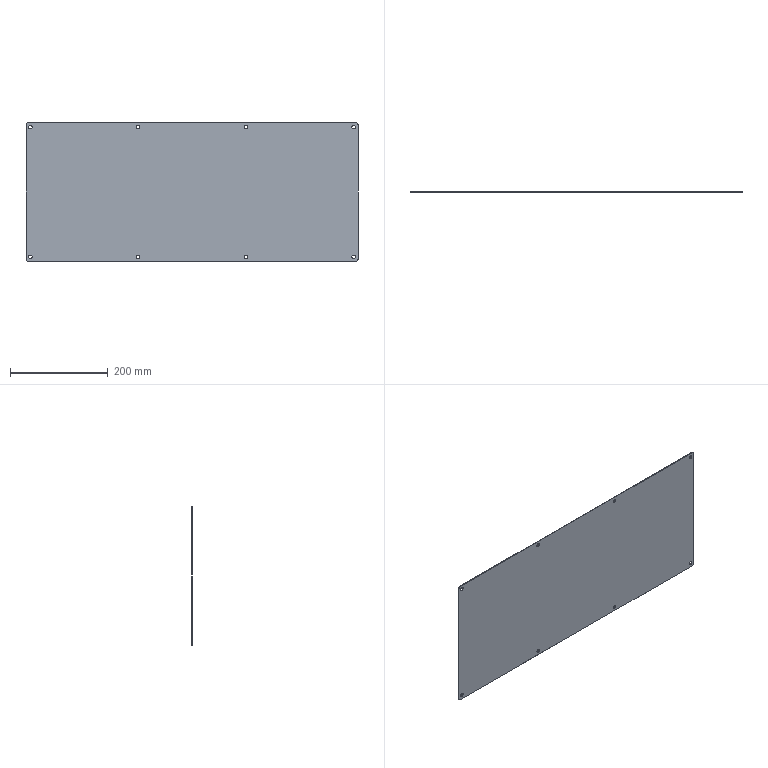Part | NX | features solid 2 | 1 solid | 26 faces | box 678 x 1.5 x 283 mm | volume 287329 mm3 | cylinder 20 | plane 6 | commonest cylinder face diameters 7 x16 8 x4
STEP:
#1=CARTESIAN_POINT('',(-330.,-1319.5,-521.5));
#2=VERTEX_POINT('',#1);
#3=CARTESIAN_POINT('',(-330.,-1318.,-521.5));
#4=VERTEX_POINT('',#3);
#5=CARTESIAN_POINT('',(-330.,-584.806,-521.5));
#6=DIRECTION('',(0.,-1.,0.));
#7=VECTOR('',#6,1000.);
#8=LINE('',#5,#7);
#9=EDGE_CURVE('',#2,#4,#8,.F.);
#10=ORIENTED_EDGE('',*,*,#9,.T.);
#11=CARTESIAN_POINT('',(-330.,-1318.,-528.5));
#12=VERTEX_POINT('',#11);
#13=CARTESIAN_POINT('',(-330.,-1318.,-525.));
#14=DIRECTION('',(0.,1.,0.));
#15=DIRECTION('',(0.,0.,1.));
#16=AXIS2_PLACEMENT_3D('',#13,#14,#15);
#17=CIRCLE('',#16,3.5);
#18=EDGE_CURVE('',#4,#12,#17,.T.);
#19=ORIENTED_EDGE('',*,*,#18,.T.);
#20=CARTESIAN_POINT('',(-330.,-1319.5,-528.5));
#21=VERTEX_POINT('',#20);
#22=CARTESIAN_POINT('',(-330.,-584.806,-528.5));
#23=DIRECTION('',(0.,-1.,0.));
#24=VECTOR('',#23,1000.);
#25=LINE('',#22,#24);
#26=EDGE_CURVE('',#12,#21,#25,.T.);
#27=ORIENTED_EDGE('',*,*,#26,.T.);
#28=CARTESIAN_POINT('',(-330.,-1319.5,-525.));
#29=DIRECTION('',(0.,-1.,0.));
#30=DIRECTION('',(1.,0.,0.));
#31=AXIS2_PLACEMENT_3D('',#28,#29,#30);
#32=CIRCLE('',#31,3.5);
#33=EDGE_CURVE('',#21,#2,#32,.T.);
#34=ORIENTED_EDGE('',*,*,#33,.T.);
#35=EDGE_LOOP('',(#10,#19,#27,#34));
#36=FACE_BOUND('',#35,.T.);
#37=CARTESIAN_POINT('',(-330.,-584.806,-525.));
#38=DIRECTION('',(0.,-1.,0.));
#39=DIRECTION('',(0.,0.,-1.));
#40=AXIS2_PLACEMENT_3D('',#37,#38,#39);
#41=CYLINDRICAL_SURFACE('',#40,3.5);
#42=ADVANCED_FACE('',(#36),#41,.F.);
#43=CARTESIAN_POINT('',(-110.,-1318.,-521.5));
#44=VERTEX_POINT('',#43);
#45=CARTESIAN_POINT('',(-110.,-1319.5,-521.5));
#46=VERTEX_POINT('',#45);
#47=CARTESIAN_POINT('',(-110.,-584.806,-521.5));
#48=DIRECTION('',(0.,-1.,0.));
#49=VECTOR('',#48,1000.);
#50=LINE('',#47,#49);
#51=EDGE_CURVE('',#44,#46,#50,.T.);
#52=ORIENTED_EDGE('',*,*,#51,.F.);
#53=CARTESIAN_POINT('',(-110.,-1318.,-528.5));
#54=VERTEX_POINT('',#53);
#55=CARTESIAN_POINT('',(-110.,-1318.,-525.));
#56=DIRECTION('',(0.,1.,0.));
#57=DIRECTION('',(0.,0.,1.));
#58=AXIS2_PLACEMENT_3D('',#55,#56,#57);
#59=CIRCLE('',#58,3.5);
#60=EDGE_CURVE('',#44,#54,#59,.T.);
#61=ORIENTED_EDGE('',*,*,#60,.T.);
#62=CARTESIAN_POINT('',(-110.,-1319.5,-528.5));
#63=VERTEX_POINT('',#62);
#64=CARTESIAN_POINT('',(-110.,-584.806,-528.5));
#65=DIRECTION('',(0.,-1.,0.));
#66=VECTOR('',#65,1000.);
#67=LINE('',#64,#66);
#68=EDGE_CURVE('',#63,#54,#67,.F.);
#69=ORIENTED_EDGE('',*,*,#68,.F.);
#70=CARTESIAN_POINT('',(-110.,-1319.5,-525.));
#71=DIRECTION('',(0.,-1.,0.));
#72=DIRECTION('',(1.,0.,0.));
#73=AXIS2_PLACEMENT_3D('',#70,#71,#72);
#74=CIRCLE('',#73,3.5);
#75=EDGE_CURVE('',#63,#46,#74,.T.);
#76=ORIENTED_EDGE('',*,*,#75,.T.);
#77=EDGE_LOOP('',(#52,#61,#69,#76));
#78=FACE_BOUND('',#77,.T.);
#79=CARTESIAN_POINT('',(-110.,-584.806,-525.));
#80=DIRECTION('',(0.,-1.,0.));
#81=DIRECTION('',(0.,0.,-1.));
#82=AXIS2_PLACEMENT_3D('',#79,#80,#81);
#83=CYLINDRICAL_SURFACE('',#82,3.5);
#84=ADVANCED_FACE('',(#78),#83,.F.);
#85=CARTESIAN_POINT('',(110.,-1318.,-521.5));
#86=VERTEX_POINT('',#85);
#87=CARTESIAN_POINT('',(110.,-1319.5,-521.5));
#88=VERTEX_POINT('',#87);
#89=CARTESIAN_POINT('',(110.,-584.806,-521.5));
#90=DIRECTION('',(0.,-1.,0.));
#91=VECTOR('',#90,1000.);
#92=LINE('',#89,#91);
#93=EDGE_CURVE('',#86,#88,#92,.T.);
#94=ORIENTED_EDGE('',*,*,#93,.F.);
#95=CARTESIAN_POINT('',(110.,-1318.,-528.5));
#96=VERTEX_POINT('',#95);
#97=CARTESIAN_POINT('',(110.,-1318.,-525.));
#98=DIRECTION('',(0.,1.,0.));
#99=DIRECTION('',(0.,0.,1.));
#100=AXIS2_PLACEMENT_3D('',#97,#98,#99);
#101=CIRCLE('',#100,3.5);
#102=EDGE_CURVE('',#86,#96,#101,.T.);
#103=ORIENTED_EDGE('',*,*,#102,.T.);
#104=CARTESIAN_POINT('',(110.,-1319.5,-528.5));
#105=VERTEX_POINT('',#104);
#106=CARTESIAN_POINT('',(110.,-584.806,-528.5));
#107=DIRECTION('',(0.,-1.,0.));
#108=VECTOR('',#107,1000.);
#109=LINE('',#106,#108);
#110=EDGE_CURVE('',#105,#96,#109,.F.);
#111=ORIENTED_EDGE('',*,*,#110,.F.);
#112=CARTESIAN_POINT('',(110.,-1319.5,-525.));
#113=DIRECTION('',(0.,-1.,0.));
#114=DIRECTION('',(1.,0.,0.));
#115=AXIS2_PLACEMENT_3D('',#112,#113,#114);
#116=CIRCLE('',#115,3.5);
#117=EDGE_CURVE('',#105,#88,#116,.T.);
#118=ORIENTED_EDGE('',*,*,#117,.T.);
#119=EDGE_LOOP('',(#94,#103,#111,#118));
#120=FACE_BOUND('',#119,.T.);
#121=CARTESIAN_POINT('',(110.,-584.806,-525.));
#122=DIRECTION('',(0.,-1.,0.));
#123=DIRECTION('',(0.,0.,-1.));
#124=AXIS2_PLACEMENT_3D('',#121,#122,#123);
#125=CYLINDRICAL_SURFACE('',#124,3.5);
#126=ADVANCED_FACE('',(#120),#125,.F.);
#127=CARTESIAN_POINT('',(330.,-1318.,-521.5));
#128=VERTEX_POINT('',#127);
#129=CARTESIAN_POINT('',(330.,-1319.5,-521.5));
#130=VERTEX_POINT('',#129);
#131=CARTESIAN_POINT('',(330.,-584.806,-521.5));
#132=DIRECTION('',(0.,-1.,0.));
#133=VECTOR('',#132,1000.);
#134=LINE('',#131,#133);
#135=EDGE_CURVE('',#128,#130,#134,.T.);
#136=ORIENTED_EDGE('',*,*,#135,.F.);
#137=CARTESIAN_POINT('',(330.,-1318.,-528.5));
#138=VERTEX_POINT('',#137);
#139=CARTESIAN_POINT('',(330.,-1318.,-525.));
#140=DIRECTION('',(0.,1.,0.));
#141=DIRECTION('',(0.,0.,1.));
#142=AXIS2_PLACEMENT_3D('',#139,#140,#141);
#143=CIRCLE('',#142,3.5);
#144=EDGE_CURVE('',#128,#138,#143,.T.);
#145=ORIENTED_EDGE('',*,*,#144,.T.);
#146=CARTESIAN_POINT('',(330.,-1319.5,-528.5));
#147=VERTEX_POINT('',#146);
#148=CARTESIAN_POINT('',(330.,-584.806,-528.5));
#149=DIRECTION('',(0.,-1.,0.));
#150=VECTOR('',#149,1000.);
#151=LINE('',#148,#150);
#152=EDGE_CURVE('',#147,#138,#151,.F.);
#153=ORIENTED_EDGE('',*,*,#152,.F.);
#154=CARTESIAN_POINT('',(330.,-1319.5,-525.));
#155=DIRECTION('',(0.,-1.,0.));
#156=DIRECTION('',(1.,0.,0.));
#157=AXIS2_PLACEMENT_3D('',#154,#155,#156);
#158=CIRCLE('',#157,3.5);
#159=EDGE_CURVE('',#147,#130,#158,.T.);
#160=ORIENTED_EDGE('',*,*,#159,.T.);
#161=EDGE_LOOP('',(#136,#145,#153,#160));
#162=FACE_BOUND('',#161,.T.);
#163=CARTESIAN_POINT('',(330.,-584.806,-525.));
#164=DIRECTION('',(0.,-1.,0.));
#165=DIRECTION('',(0.,0.,-1.));
#166=AXIS2_PLACEMENT_3D('',#163,#164,#165);
#167=CYLINDRICAL_SURFACE('',#166,3.5);
#168=ADVANCED_FACE('',(#162),#167,.F.);
#169=CARTESIAN_POINT('',(330.,-1318.,-256.5));
#170=VERTEX_POINT('',#169);
#171=CARTESIAN_POINT('',(330.,-1319.5,-256.5));
#172=VERTEX_POINT('',#171);
#173=CARTESIAN_POINT('',(330.,-584.806,-256.5));
#174=DIRECTION('',(0.,-1.,0.));
#175=VECTOR('',#174,1000.);
#176=LINE('',#173,#175);
#177=EDGE_CURVE('',#170,#172,#176,.T.);
#178=ORIENTED_EDGE('',*,*,#177,.F.);
#179=CARTESIAN_POINT('',(330.,-1318.,-263.5));
#180=VERTEX_POINT('',#179);
#181=CARTESIAN_POINT('',(330.,-1318.,-260.));
#182=DIRECTION('',(0.,1.,0.));
#183=DIRECTION('',(0.,0.,1.));
#184=AXIS2_PLACEMENT_3D('',#181,#182,#183);
#185=CIRCLE('',#184,3.5);
#186=EDGE_CURVE('',#170,#180,#185,.T.);
#187=ORIENTED_EDGE('',*,*,#186,.T.);
#188=CARTESIAN_POINT('',(330.,-1319.5,-263.5));
#189=VERTEX_POINT('',#188);
#190=CARTESIAN_POINT('',(330.,-584.806,-263.5));
#191=DIRECTION('',(0.,-1.,0.));
#192=VECTOR('',#191,1000.);
#193=LINE('',#190,#192);
#194=EDGE_CURVE('',#189,#180,#193,.F.);
#195=ORIENTED_EDGE('',*,*,#194,.F.);
#196=CARTESIAN_POINT('',(330.,-1319.5,-260.));
#197=DIRECTION('',(0.,-1.,0.));
#198=DIRECTION('',(1.,0.,0.));
#199=AXIS2_PLACEMENT_3D('',#196,#197,#198);
#200=CIRCLE('',#199,3.5);
#201=EDGE_CURVE('',#189,#172,#200,.T.);
#202=ORIENTED_EDGE('',*,*,#201,.T.);
#203=EDGE_LOOP('',(#178,#187,#195,#202));
#204=FACE_BOUND('',#203,.T.);
#205=CARTESIAN_POINT('',(330.,-584.806,-260.));
#206=DIRECTION('',(0.,-1.,0.));
#207=DIRECTION('',(0.,0.,-1.));
#208=AXIS2_PLACEMENT_3D('',#205,#206,#207);
#209=CYLINDRICAL_SURFACE('',#208,3.5);
#210=ADVANCED_FACE('',(#204),#209,.F.);
#211=CARTESIAN_POINT('',(110.,-1319.5,-256.5));
#212=VERTEX_POINT('',#211);
#213=CARTESIAN_POINT('',(110.,-1318.,-256.5));
#214=VERTEX_POINT('',#213);
#215=CARTESIAN_POINT('',(110.,-584.806,-256.5));
#216=DIRECTION('',(0.,-1.,0.));
#217=VECTOR('',#216,1000.);
#218=LINE('',#215,#217);
#219=EDGE_CURVE('',#212,#214,#218,.F.);
#220=ORIENTED_EDGE('',*,*,#219,.T.);
#221=CARTESIAN_POINT('',(110.,-1318.,-263.5));
#222=VERTEX_POINT('',#221);
#223=CARTESIAN_POINT('',(110.,-1318.,-260.));
#224=DIRECTION('',(0.,1.,0.));
#225=DIRECTION('',(0.,0.,1.));
#226=AXIS2_PLACEMENT_3D('',#223,#224,#225);
#227=CIRCLE('',#226,3.5);
#228=EDGE_CURVE('',#214,#222,#227,.T.);
#229=ORIENTED_EDGE('',*,*,#228,.T.);
#230=CARTESIAN_POINT('',(110.,-1319.5,-263.5));
#231=VERTEX_POINT('',#230);
#232=CARTESIAN_POINT('',(110.,-584.806,-263.5));
#233=DIRECTION('',(0.,-1.,0.));
#234=VECTOR('',#233,1000.);
#235=LINE('',#232,#234);
#236=EDGE_CURVE('',#222,#231,#235,.T.);
#237=ORIENTED_EDGE('',*,*,#236,.T.);
#238=CARTESIAN_POINT('',(110.,-1319.5,-260.));
#239=DIRECTION('',(0.,-1.,0.));
#240=DIRECTION('',(1.,0.,0.));
#241=AXIS2_PLACEMENT_3D('',#238,#239,#240);
#242=CIRCLE('',#241,3.5);
#243=EDGE_CURVE('',#231,#212,#242,.T.);
#244=ORIENTED_EDGE('',*,*,#243,.T.);
#245=EDGE_LOOP('',(#220,#229,#237,#244));
#246=FACE_BOUND('',#245,.T.);
#247=CARTESIAN_POINT('',(110.,-584.806,-260.));
#248=DIRECTION('',(0.,-1.,0.));
#249=DIRECTION('',(0.,0.,-1.));
#250=AXIS2_PLACEMENT_3D('',#247,#248,#249);
#251=CYLINDRICAL_SURFACE('',#250,3.5);
#252=ADVANCED_FACE('',(#246),#251,.F.);
#253=CARTESIAN_POINT('',(-110.,-1318.,-256.5));
#254=VERTEX_POINT('',#253);
#255=CARTESIAN_POINT('',(-110.,-1319.5,-256.5));
#256=VERTEX_POINT('',#255);
#257=CARTESIAN_POINT('',(-110.,-584.806,-256.5));
#258=DIRECTION('',(0.,-1.,0.));
#259=VECTOR('',#258,1000.);
#260=LINE('',#257,#259);
#261=EDGE_CURVE('',#254,#256,#260,.T.);
#262=ORIENTED_EDGE('',*,*,#261,.F.);
#263=CARTESIAN_POINT('',(-110.,-1318.,-263.5));
#264=VERTEX_POINT('',#263);
#265=CARTESIAN_POINT('',(-110.,-1318.,-260.));
#266=DIRECTION('',(0.,1.,0.));
#267=DIRECTION('',(0.,0.,1.));
#268=AXIS2_PLACEMENT_3D('',#265,#266,#267);
#269=CIRCLE('',#268,3.5);
#270=EDGE_CURVE('',#254,#264,#269,.T.);
#271=ORIENTED_EDGE('',*,*,#270,.T.);
#272=CARTESIAN_POINT('',(-110.,-1319.5,-263.5));
#273=VERTEX_POINT('',#272);
#274=CARTESIAN_POINT('',(-110.,-584.806,-263.5));
#275=DIRECTION('',(0.,-1.,0.));
#276=VECTOR('',#275,1000.);
#277=LINE('',#274,#276);
#278=EDGE_CURVE('',#273,#264,#277,.F.);
#279=ORIENTED_EDGE('',*,*,#278,.F.);
#280=CARTESIAN_POINT('',(-110.,-1319.5,-260.));
#281=DIRECTION('',(0.,-1.,0.));
#282=DIRECTION('',(1.,0.,0.));
#283=AXIS2_PLACEMENT_3D('',#280,#281,#282);
#284=CIRCLE('',#283,3.5);
#285=EDGE_CURVE('',#273,#256,#284,.T.);
#286=ORIENTED_EDGE('',*,*,#285,.T.);
#287=EDGE_LOOP('',(#262,#271,#279,#286));
#288=FACE_BOUND('',#287,.T.);
#289=CARTESIAN_POINT('',(-110.,-584.806,-260.));
#290=DIRECTION('',(0.,-1.,0.));
#291=DIRECTION('',(0.,0.,-1.));
#292=AXIS2_PLACEMENT_3D('',#289,#290,#291);
#293=CYLINDRICAL_SURFACE('',#292,3.5);
#294=ADVANCED_FACE('',(#288),#293,.F.);
#295=CARTESIAN_POINT('',(-330.,-1318.,-256.5));
#296=VERTEX_POINT('',#295);
#297=CARTESIAN_POINT('',(-330.,-1319.5,-256.5));
#298=VERTEX_POINT('',#297);
#299=CARTESIAN_POINT('',(-330.,-584.806,-256.5));
#300=DIRECTION('',(0.,-1.,0.));
#301=VECTOR('',#300,1000.);
#302=LINE('',#299,#301);
#303=EDGE_CURVE('',#296,#298,#302,.T.);
#304=ORIENTED_EDGE('',*,*,#303,.F.);
#305=CARTESIAN_POINT('',(-330.,-1318.,-263.5));
#306=VERTEX_POINT('',#305);
#307=CARTESIAN_POINT('',(-330.,-1318.,-260.));
#308=DIRECTION('',(0.,1.,0.));
#309=DIRECTION('',(0.,0.,1.));
#310=AXIS2_PLACEMENT_3D('',#307,#308,#309);
#311=CIRCLE('',#310,3.5);
#312=EDGE_CURVE('',#296,#306,#311,.T.);
#313=ORIENTED_EDGE('',*,*,#312,.T.);
#314=CARTESIAN_POINT('',(-330.,-1319.5,-263.5));
#315=VERTEX_POINT('',#314);
#316=CARTESIAN_POINT('',(-330.,-584.806,-263.5));
#317=DIRECTION('',(0.,-1.,0.));
#318=VECTOR('',#317,1000.);
#319=LINE('',#316,#318);
#320=EDGE_CURVE('',#315,#306,#319,.F.);
#321=ORIENTED_EDGE('',*,*,#320,.F.);
#322=CARTESIAN_POINT('',(-330.,-1319.5,-260.));
#323=DIRECTION('',(0.,-1.,0.));
#324=DIRECTION('',(1.,0.,0.));
#325=AXIS2_PLACEMENT_3D('',#322,#323,#324);
#326=CIRCLE('',#325,3.5);
#327=EDGE_CURVE('',#315,#298,#326,.T.);
#328=ORIENTED_EDGE('',*,*,#327,.T.);
#329=EDGE_LOOP('',(#304,#313,#321,#328));
#330=FACE_BOUND('',#329,.T.);
#331=CARTESIAN_POINT('',(-330.,-584.806,-260.));
#332=DIRECTION('',(0.,-1.,0.));
#333=DIRECTION('',(0.,0.,-1.));
#334=AXIS2_PLACEMENT_3D('',#331,#332,#333);
#335=CYLINDRICAL_SURFACE('',#334,3.5);
#336=ADVANCED_FACE('',(#330),#335,.F.);
#337=ORIENTED_EDGE('',*,*,#327,.F.);
#338=CARTESIAN_POINT('',(-330.,-1319.5,-260.));
#339=DIRECTION('',(0.,-1.,0.));
#340=DIRECTION('',(1.,0.,0.));
#341=AXIS2_PLACEMENT_3D('',#338,#339,#340);
#342=CIRCLE('',#341,3.5);
#343=EDGE_CURVE('',#298,#315,#342,.T.);
#344=ORIENTED_EDGE('',*,*,#343,.F.);
#345=EDGE_LOOP('',(#337,#344));
#346=FACE_BOUND('',#345,.T.);
#347=ORIENTED_EDGE('',*,*,#285,.F.);
#348=CARTESIAN_POINT('',(-110.,-1319.5,-260.));
#349=DIRECTION('',(0.,-1.,0.));
#350=DIRECTION('',(1.,0.,0.));
#351=AXIS2_PLACEMENT_3D('',#348,#349,#350);
#352=CIRCLE('',#351,3.5);
#353=EDGE_CURVE('',#256,#273,#352,.T.);
#354=ORIENTED_EDGE('',*,*,#353,.F.);
#355=EDGE_LOOP('',(#347,#354));
#356=FACE_BOUND('',#355,.T.);
#357=ORIENTED_EDGE('',*,*,#243,.F.);
#358=CARTESIAN_POINT('',(110.,-1319.5,-260.));
#359=DIRECTION('',(0.,-1.,0.));
#360=DIRECTION('',(1.,0.,0.));
#361=AXIS2_PLACEMENT_3D('',#358,#359,#360);
#362=CIRCLE('',#361,3.5);
#363=EDGE_CURVE('',#212,#231,#362,.T.);
#364=ORIENTED_EDGE('',*,*,#363,.F.);
#365=EDGE_LOOP('',(#357,#364));
#366=FACE_BOUND('',#365,.T.);
#367=ORIENTED_EDGE('',*,*,#201,.F.);
#368=CARTESIAN_POINT('',(330.,-1319.5,-260.));
#369=DIRECTION('',(0.,-1.,0.));
#370=DIRECTION('',(1.,0.,0.));
#371=AXIS2_PLACEMENT_3D('',#368,#369,#370);
#372=CIRCLE('',#371,3.5);
#373=EDGE_CURVE('',#172,#189,#372,.T.);
#374=ORIENTED_EDGE('',*,*,#373,.F.);
#375=EDGE_LOOP('',(#367,#374));
#376=FACE_BOUND('',#375,.T.);
#377=ORIENTED_EDGE('',*,*,#159,.F.);
#378=CARTESIAN_POINT('',(330.,-1319.5,-525.));
#379=DIRECTION('',(0.,-1.,0.));
#380=DIRECTION('',(1.,0.,0.));
#381=AXIS2_PLACEMENT_3D('',#378,#379,#380);
#382=CIRCLE('',#381,3.5);
#383=EDGE_CURVE('',#130,#147,#382,.T.);
#384=ORIENTED_EDGE('',*,*,#383,.F.);
#385=EDGE_LOOP('',(#377,#384));
#386=FACE_BOUND('',#385,.T.);
#387=ORIENTED_EDGE('',*,*,#117,.F.);
#388=CARTESIAN_POINT('',(110.,-1319.5,-525.));
#389=DIRECTION('',(0.,-1.,0.));
#390=DIRECTION('',(1.,0.,0.));
#391=AXIS2_PLACEMENT_3D('',#388,#389,#390);
#392=CIRCLE('',#391,3.5);
#393=EDGE_CURVE('',#88,#105,#392,.T.);
#394=ORIENTED_EDGE('',*,*,#393,.F.);
#395=EDGE_LOOP('',(#387,#394));
#396=FACE_BOUND('',#395,.T.);
#397=ORIENTED_EDGE('',*,*,#75,.F.);
#398=CARTESIAN_POINT('',(-110.,-1319.5,-525.));
#399=DIRECTION('',(0.,-1.,0.));
#400=DIRECTION('',(1.,0.,0.));
#401=AXIS2_PLACEMENT_3D('',#398,#399,#400);
#402=CIRCLE('',#401,3.5);
#403=EDGE_CURVE('',#46,#63,#402,.T.);
#404=ORIENTED_EDGE('',*,*,#403,.F.);
#405=EDGE_LOOP('',(#397,#404));
#406=FACE_BOUND('',#405,.T.);
#407=ORIENTED_EDGE('',*,*,#33,.F.);
#408=CARTESIAN_POINT('',(-330.,-1319.5,-525.));
#409=DIRECTION('',(0.,-1.,0.));
#410=DIRECTION('',(1.,0.,0.));
#411=AXIS2_PLACEMENT_3D('',#408,#409,#410);
#412=CIRCLE('',#411,3.5);
#413=EDGE_CURVE('',#2,#21,#412,.T.);
#414=ORIENTED_EDGE('',*,*,#413,.F.);
#415=EDGE_LOOP('',(#407,#414));
#416=FACE_BOUND('',#415,.T.);
#417=CARTESIAN_POINT('',(-339.,-1319.5,-255.));
#418=VERTEX_POINT('',#417);
#419=CARTESIAN_POINT('',(-335.,-1319.5,-251.));
#420=VERTEX_POINT('',#419);
#421=CARTESIAN_POINT('',(-335.,-1319.5,-255.));
#422=DIRECTION('',(0.,1.,0.));
#423=DIRECTION('',(1.,0.,0.));
#424=AXIS2_PLACEMENT_3D('',#421,#422,#423);
#425=CIRCLE('',#424,4.);
#426=EDGE_CURVE('',#418,#420,#425,.T.);
#427=ORIENTED_EDGE('',*,*,#426,.F.);
#428=CARTESIAN_POINT('',(-339.,-1319.5,-530.));
#429=VERTEX_POINT('',#428);
#430=CARTESIAN_POINT('',(-339.,-1319.5,-530.));
#431=DIRECTION('',(0.,0.,1.));
#432=VECTOR('',#431,1000.);
#433=LINE('',#430,#432);
#434=EDGE_CURVE('',#429,#418,#433,.T.);
#435=ORIENTED_EDGE('',*,*,#434,.F.);
#436=CARTESIAN_POINT('',(-335.,-1319.5,-534.));
#437=VERTEX_POINT('',#436);
#438=CARTESIAN_POINT('',(-335.,-1319.5,-530.));
#439=DIRECTION('',(0.,1.,0.));
#440=DIRECTION('',(1.,0.,0.));
#441=AXIS2_PLACEMENT_3D('',#438,#439,#440);
#442=CIRCLE('',#441,4.);
#443=EDGE_CURVE('',#437,#429,#442,.T.);
#444=ORIENTED_EDGE('',*,*,#443,.F.);
#445=CARTESIAN_POINT('',(335.,-1319.5,-534.));
#446=VERTEX_POINT('',#445);
#447=CARTESIAN_POINT('',(335.,-1319.5,-534.));
#448=DIRECTION('',(-1.,0.,0.));
#449=VECTOR('',#448,1000.);
#450=LINE('',#447,#449);
#451=EDGE_CURVE('',#446,#437,#450,.T.);
#452=ORIENTED_EDGE('',*,*,#451,.F.);
#453=CARTESIAN_POINT('',(339.,-1319.5,-530.));
#454=VERTEX_POINT('',#453);
#455=CARTESIAN_POINT('',(335.,-1319.5,-530.));
#456=DIRECTION('',(0.,1.,0.));
#457=DIRECTION('',(1.,0.,0.));
#458=AXIS2_PLACEMENT_3D('',#455,#456,#457);
#459=CIRCLE('',#458,4.);
#460=EDGE_CURVE('',#454,#446,#459,.T.);
#461=ORIENTED_EDGE('',*,*,#460,.F.);
#462=CARTESIAN_POINT('',(339.,-1319.5,-255.));
#463=VERTEX_POINT('',#462);
#464=CARTESIAN_POINT('',(339.,-1319.5,-255.));
#465=DIRECTION('',(0.,0.,-1.));
#466=VECTOR('',#465,1000.);
#467=LINE('',#464,#466);
#468=EDGE_CURVE('',#463,#454,#467,.T.);
#469=ORIENTED_EDGE('',*,*,#468,.F.);
#470=CARTESIAN_POINT('',(335.,-1319.5,-251.));
#471=VERTEX_POINT('',#470);
#472=CARTESIAN_POINT('',(335.,-1319.5,-255.));
#473=DIRECTION('',(0.,1.,0.));
#474=DIRECTION('',(-1.,0.,0.));
#475=AXIS2_PLACEMENT_3D('',#472,#473,#474);
#476=CIRCLE('',#475,4.);
#477=EDGE_CURVE('',#471,#463,#476,.T.);
#478=ORIENTED_EDGE('',*,*,#477,.F.);
#479=CARTESIAN_POINT('',(-335.,-1319.5,-251.));
#480=DIRECTION('',(1.,0.,0.));
#481=VECTOR('',#480,1000.);
#482=LINE('',#479,#481);
#483=EDGE_CURVE('',#420,#471,#482,.T.);
#484=ORIENTED_EDGE('',*,*,#483,.F.);
#485=EDGE_LOOP('',(#427,#435,#444,#452,#461,#469,#478,#484));
#486=FACE_BOUND('',#485,.T.);
#487=CARTESIAN_POINT('',(-335.,-1319.5,-255.));
#488=DIRECTION('',(0.,1.,0.));
#489=DIRECTION('',(1.,0.,0.));
#490=AXIS2_PLACEMENT_3D('',#487,#488,#489);
#491=PLANE('',#490);
#492=ADVANCED_FACE('',(#346,#356,#366,#376,#386,#396,#406,#416,#486),#491,.F.);
#493=CARTESIAN_POINT('',(-330.,-1318.,-260.));
#494=DIRECTION('',(0.,1.,0.));
#495=DIRECTION('',(0.,0.,1.));
#496=AXIS2_PLACEMENT_3D('',#493,#494,#495);
#497=CIRCLE('',#496,3.5);
#498=EDGE_CURVE('',#306,#296,#497,.T.);
#499=ORIENTED_EDGE('',*,*,#498,.F.);
#500=ORIENTED_EDGE('',*,*,#312,.F.);
#501=EDGE_LOOP('',(#499,#500));
#502=FACE_BOUND('',#501,.T.);
#503=CARTESIAN_POINT('',(-110.,-1318.,-260.));
#504=DIRECTION('',(0.,1.,0.));
#505=DIRECTION('',(0.,0.,1.));
#506=AXIS2_PLACEMENT_3D('',#503,#504,#505);
#507=CIRCLE('',#506,3.5);
#508=EDGE_CURVE('',#264,#254,#507,.T.);
#509=ORIENTED_EDGE('',*,*,#508,.F.);
#510=ORIENTED_EDGE('',*,*,#270,.F.);
#511=EDGE_LOOP('',(#509,#510));
#512=FACE_BOUND('',#511,.T.);
#513=CARTESIAN_POINT('',(110.,-1318.,-260.));
#514=DIRECTION('',(0.,1.,0.));
#515=DIRECTION('',(0.,0.,1.));
#516=AXIS2_PLACEMENT_3D('',#513,#514,#515);
#517=CIRCLE('',#516,3.5);
#518=EDGE_CURVE('',#222,#214,#517,.T.);
#519=ORIENTED_EDGE('',*,*,#518,.F.);
#520=ORIENTED_EDGE('',*,*,#228,.F.);
#521=EDGE_LOOP('',(#519,#520));
#522=FACE_BOUND('',#521,.T.);
#523=CARTESIAN_POINT('',(330.,-1318.,-260.));
#524=DIRECTION('',(0.,1.,0.));
#525=DIRECTION('',(0.,0.,1.));
#526=AXIS2_PLACEMENT_3D('',#523,#524,#525);
#527=CIRCLE('',#526,3.5);
#528=EDGE_CURVE('',#180,#170,#527,.T.);
#529=ORIENTED_EDGE('',*,*,#528,.F.);
#530=ORIENTED_EDGE('',*,*,#186,.F.);
#531=EDGE_LOOP('',(#529,#530));
#532=FACE_BOUND('',#531,.T.);
#533=CARTESIAN_POINT('',(330.,-1318.,-525.));
#534=DIRECTION('',(0.,1.,0.));
#535=DIRECTION('',(0.,0.,1.));
#536=AXIS2_PLACEMENT_3D('',#533,#534,#535);
#537=CIRCLE('',#536,3.5);
#538=EDGE_CURVE('',#138,#128,#537,.T.);
#539=ORIENTED_EDGE('',*,*,#538,.F.);
#540=ORIENTED_EDGE('',*,*,#144,.F.);
#541=EDGE_LOOP('',(#539,#540));
#542=FACE_BOUND('',#541,.T.);
#543=CARTESIAN_POINT('',(110.,-1318.,-525.));
#544=DIRECTION('',(0.,1.,0.));
#545=DIRECTION('',(0.,0.,1.));
#546=AXIS2_PLACEMENT_3D('',#543,#544,#545);
#547=CIRCLE('',#546,3.5);
#548=EDGE_CURVE('',#96,#86,#547,.T.);
#549=ORIENTED_EDGE('',*,*,#548,.F.);
#550=ORIENTED_EDGE('',*,*,#102,.F.);
#551=EDGE_LOOP('',(#549,#550));
#552=FACE_BOUND('',#551,.T.);
#553=CARTESIAN_POINT('',(-110.,-1318.,-525.));
#554=DIRECTION('',(0.,1.,0.));
#555=DIRECTION('',(0.,0.,1.));
#556=AXIS2_PLACEMENT_3D('',#553,#554,#555);
#557=CIRCLE('',#556,3.5);
#558=EDGE_CURVE('',#54,#44,#557,.T.);
#559=ORIENTED_EDGE('',*,*,#558,.F.);
#560=ORIENTED_EDGE('',*,*,#60,.F.);
#561=EDGE_LOOP('',(#559,#560));
#562=FACE_BOUND('',#561,.T.);
#563=CARTESIAN_POINT('',(-330.,-1318.,-525.));
#564=DIRECTION('',(0.,1.,0.));
#565=DIRECTION('',(0.,0.,1.));
#566=AXIS2_PLACEMENT_3D('',#563,#564,#565);
#567=CIRCLE('',#566,3.5);
#568=EDGE_CURVE('',#12,#4,#567,.T.);
#569=ORIENTED_EDGE('',*,*,#568,.F.);
#570=ORIENTED_EDGE('',*,*,#18,.F.);
#571=EDGE_LOOP('',(#569,#570));
#572=FACE_BOUND('',#571,.T.);
#573=CARTESIAN_POINT('',(-339.,-1318.,-255.));
#574=VERTEX_POINT('',#573);
#575=CARTESIAN_POINT('',(-335.,-1318.,-251.));
#576=VERTEX_POINT('',#575);
#577=CARTESIAN_POINT('',(-335.,-1318.,-255.));
#578=DIRECTION('',(0.,1.,0.));
#579=DIRECTION('',(1.,0.,0.));
#580=AXIS2_PLACEMENT_3D('',#577,#578,#579);
#581=CIRCLE('',#580,4.);
#582=EDGE_CURVE('',#574,#576,#581,.T.);
#583=ORIENTED_EDGE('',*,*,#582,.T.);
#584=CARTESIAN_POINT('',(335.,-1318.,-251.));
#585=VERTEX_POINT('',#584);
#586=CARTESIAN_POINT('',(-335.,-1318.,-251.));
#587=DIRECTION('',(1.,0.,0.));
#588=VECTOR('',#587,1000.);
#589=LINE('',#586,#588);
#590=EDGE_CURVE('',#576,#585,#589,.T.);
#591=ORIENTED_EDGE('',*,*,#590,.T.);
#592=CARTESIAN_POINT('',(339.,-1318.,-255.));
#593=VERTEX_POINT('',#592);
#594=CARTESIAN_POINT('',(335.,-1318.,-255.));
#595=DIRECTION('',(0.,1.,0.));
#596=DIRECTION('',(-1.,0.,0.));
#597=AXIS2_PLACEMENT_3D('',#594,#595,#596);
#598=CIRCLE('',#597,4.);
#599=EDGE_CURVE('',#585,#593,#598,.T.);
#600=ORIENTED_EDGE('',*,*,#599,.T.);
#601=CARTESIAN_POINT('',(339.,-1318.,-530.));
#602=VERTEX_POINT('',#601);
#603=CARTESIAN_POINT('',(339.,-1318.,-255.));
#604=DIRECTION('',(0.,0.,-1.));
#605=VECTOR('',#604,1000.);
#606=LINE('',#603,#605);
#607=EDGE_CURVE('',#593,#602,#606,.T.);
#608=ORIENTED_EDGE('',*,*,#607,.T.);
#609=CARTESIAN_POINT('',(335.,-1318.,-534.));
#610=VERTEX_POINT('',#609);
#611=CARTESIAN_POINT('',(335.,-1318.,-530.));
#612=DIRECTION('',(0.,1.,0.));
#613=DIRECTION('',(1.,0.,0.));
#614=AXIS2_PLACEMENT_3D('',#611,#612,#613);
#615=CIRCLE('',#614,4.);
#616=EDGE_CURVE('',#602,#610,#615,.T.);
#617=ORIENTED_EDGE('',*,*,#616,.T.);
#618=CARTESIAN_POINT('',(-335.,-1318.,-534.));
#619=VERTEX_POINT('',#618);
#620=CARTESIAN_POINT('',(335.,-1318.,-534.));
#621=DIRECTION('',(-1.,0.,0.));
#622=VECTOR('',#621,1000.);
#623=LINE('',#620,#622);
#624=EDGE_CURVE('',#610,#619,#623,.T.);
#625=ORIENTED_EDGE('',*,*,#624,.T.);
#626=CARTESIAN_POINT('',(-339.,-1318.,-530.));
#627=VERTEX_POINT('',#626);
#628=CARTESIAN_POINT('',(-335.,-1318.,-530.));
#629=DIRECTION('',(0.,1.,0.));
#630=DIRECTION('',(1.,0.,0.));
#631=AXIS2_PLACEMENT_3D('',#628,#629,#630);
#632=CIRCLE('',#631,4.);
#633=EDGE_CURVE('',#619,#627,#632,.T.);
#634=ORIENTED_EDGE('',*,*,#633,.T.);
#635=CARTESIAN_POINT('',(-339.,-1318.,-530.));
#636=DIRECTION('',(0.,0.,1.));
#637=VECTOR('',#636,1000.);
#638=LINE('',#635,#637);
#639=EDGE_CURVE('',#627,#574,#638,.T.);
#640=ORIENTED_EDGE('',*,*,#639,.T.);
#641=EDGE_LOOP('',(#583,#591,#600,#608,#617,#625,#634,#640));
#642=FACE_BOUND('',#641,.T.);
#643=CARTESIAN_POINT('',(-335.,-1318.,-255.));
#644=DIRECTION('',(0.,1.,0.));
#645=DIRECTION('',(1.,0.,0.));
#646=AXIS2_PLACEMENT_3D('',#643,#644,#645);
#647=PLANE('',#646);
#648=ADVANCED_FACE('',(#502,#512,#522,#532,#542,#552,#562,#572,#642),#647,.T.);
#649=ORIENTED_EDGE('',*,*,#434,.T.);
#650=CARTESIAN_POINT('',(-339.,-1318.,-255.));
#651=DIRECTION('',(0.,-1.,0.));
#652=VECTOR('',#651,1000.);
#653=LINE('',#650,#652);
#654=EDGE_CURVE('',#574,#418,#653,.T.);
#655=ORIENTED_EDGE('',*,*,#654,.F.);
#656=ORIENTED_EDGE('',*,*,#639,.F.);
#657=CARTESIAN_POINT('',(-339.,-1318.,-530.));
#658=DIRECTION('',(0.,-1.,0.));
#659=VECTOR('',#658,1000.);
#660=LINE('',#657,#659);
#661=EDGE_CURVE('',#627,#429,#660,.T.);
#662=ORIENTED_EDGE('',*,*,#661,.T.);
#663=EDGE_LOOP('',(#649,#655,#656,#662));
#664=FACE_BOUND('',#663,.T.);
#665=CARTESIAN_POINT('',(-339.,-1318.,-530.));
#666=DIRECTION('',(1.,0.,0.));
#667=DIRECTION('',(0.,0.,1.));
#668=AXIS2_PLACEMENT_3D('',#665,#666,#667);
#669=PLANE('',#668);
#670=ADVANCED_FACE('',(#664),#669,.F.);
#671=ORIENTED_EDGE('',*,*,#443,.T.);
#672=ORIENTED_EDGE('',*,*,#661,.F.);
#673=ORIENTED_EDGE('',*,*,#633,.F.);
#674=CARTESIAN_POINT('',(-335.,-1318.,-534.));
#675=DIRECTION('',(0.,-1.,0.));
#676=VECTOR('',#675,1000.);
#677=LINE('',#674,#676);
#678=EDGE_CURVE('',#619,#437,#677,.T.);
#679=ORIENTED_EDGE('',*,*,#678,.T.);
#680=EDGE_LOOP('',(#671,#672,#673,#679));
#681=FACE_BOUND('',#680,.T.);
#682=CARTESIAN_POINT('',(-335.,-1318.,-530.));
#683=DIRECTION('',(0.,-1.,0.));
#684=DIRECTION('',(0.,0.,-1.));
#685=AXIS2_PLACEMENT_3D('',#682,#683,#684);
#686=CYLINDRICAL_SURFACE('',#685,4.);
#687=ADVANCED_FACE('',(#681),#686,.T.);
#688=ORIENTED_EDGE('',*,*,#451,.T.);
#689=ORIENTED_EDGE('',*,*,#678,.F.);
#690=ORIENTED_EDGE('',*,*,#624,.F.);
#691=CARTESIAN_POINT('',(335.,-1318.,-534.));
#692=DIRECTION('',(0.,-1.,0.));
#693=VECTOR('',#692,1000.);
#694=LINE('',#691,#693);
#695=EDGE_CURVE('',#610,#446,#694,.T.);
#696=ORIENTED_EDGE('',*,*,#695,.T.);
#697=EDGE_LOOP('',(#688,#689,#690,#696));
#698=FACE_BOUND('',#697,.T.);
#699=CARTESIAN_POINT('',(335.,-1318.,-534.));
#700=DIRECTION('',(0.,0.,1.));
#701=DIRECTION('',(1.,0.,0.));
#702=AXIS2_PLACEMENT_3D('',#699,#700,#701);
#703=PLANE('',#702);
#704=ADVANCED_FACE('',(#698),#703,.F.);
#705=ORIENTED_EDGE('',*,*,#460,.T.);
#706=ORIENTED_EDGE('',*,*,#695,.F.);
#707=ORIENTED_EDGE('',*,*,#616,.F.);
#708=CARTESIAN_POINT('',(339.,-1318.,-530.));
#709=DIRECTION('',(0.,-1.,0.));
#710=VECTOR('',#709,1000.);
#711=LINE('',#708,#710);
#712=EDGE_CURVE('',#602,#454,#711,.T.);
#713=ORIENTED_EDGE('',*,*,#712,.T.);
#714=EDGE_LOOP('',(#705,#706,#707,#713));
#715=FACE_BOUND('',#714,.T.);
#716=CARTESIAN_POINT('',(335.,-1318.,-530.));
#717=DIRECTION('',(0.,-1.,0.));
#718=DIRECTION('',(0.,0.,-1.));
#719=AXIS2_PLACEMENT_3D('',#716,#717,#718);
#720=CYLINDRICAL_SURFACE('',#719,4.);
#721=ADVANCED_FACE('',(#715),#720,.T.);
#722=ORIENTED_EDGE('',*,*,#468,.T.);
#723=ORIENTED_EDGE('',*,*,#712,.F.);
#724=ORIENTED_EDGE('',*,*,#607,.F.);
#725=CARTESIAN_POINT('',(339.,-1318.,-255.));
#726=DIRECTION('',(0.,-1.,0.));
#727=VECTOR('',#726,1000.);
#728=LINE('',#725,#727);
#729=EDGE_CURVE('',#593,#463,#728,.T.);
#730=ORIENTED_EDGE('',*,*,#729,.T.);
#731=EDGE_LOOP('',(#722,#723,#724,#730));
#732=FACE_BOUND('',#731,.T.);
#733=CARTESIAN_POINT('',(339.,-1318.,-255.));
#734=DIRECTION('',(-1.,0.,0.));
#735=DIRECTION('',(0.,0.,1.));
#736=AXIS2_PLACEMENT_3D('',#733,#734,#735);
#737=PLANE('',#736);
#738=ADVANCED_FACE('',(#732),#737,.F.);
#739=ORIENTED_EDGE('',*,*,#477,.T.);
#740=ORIENTED_EDGE('',*,*,#729,.F.);
#741=ORIENTED_EDGE('',*,*,#599,.F.);
#742=CARTESIAN_POINT('',(335.,-1318.,-251.));
#743=DIRECTION('',(0.,-1.,0.));
#744=VECTOR('',#743,1000.);
#745=LINE('',#742,#744);
#746=EDGE_CURVE('',#585,#471,#745,.T.);
#747=ORIENTED_EDGE('',*,*,#746,.T.);
#748=EDGE_LOOP('',(#739,#740,#741,#747));
#749=FACE_BOUND('',#748,.T.);
#750=CARTESIAN_POINT('',(335.,-1318.,-255.));
#751=DIRECTION('',(0.,-1.,0.));
#752=DIRECTION('',(0.,0.,-1.));
#753=AXIS2_PLACEMENT_3D('',#750,#751,#752);
#754=CYLINDRICAL_SURFACE('',#753,4.);
#755=ADVANCED_FACE('',(#749),#754,.T.);
#756=ORIENTED_EDGE('',*,*,#483,.T.);
#757=ORIENTED_EDGE('',*,*,#746,.F.);
#758=ORIENTED_EDGE('',*,*,#590,.F.);
#759=CARTESIAN_POINT('',(-335.,-1318.,-251.));
#760=DIRECTION('',(0.,-1.,0.));
#761=VECTOR('',#760,1000.);
#762=LINE('',#759,#761);
#763=EDGE_CURVE('',#576,#420,#762,.T.);
#764=ORIENTED_EDGE('',*,*,#763,.T.);
#765=EDGE_LOOP('',(#756,#757,#758,#764));
#766=FACE_BOUND('',#765,.T.);
#767=CARTESIAN_POINT('',(-335.,-1318.,-251.));
#768=DIRECTION('',(0.,0.,-1.));
#769=DIRECTION('',(0.,-1.,0.));
#770=AXIS2_PLACEMENT_3D('',#767,#768,#769);
#771=PLANE('',#770);
#772=ADVANCED_FACE('',(#766),#771,.F.);
#773=ORIENTED_EDGE('',*,*,#426,.T.);
#774=ORIENTED_EDGE('',*,*,#763,.F.);
#775=ORIENTED_EDGE('',*,*,#582,.F.);
#776=ORIENTED_EDGE('',*,*,#654,.T.);
#777=EDGE_LOOP('',(#773,#774,#775,#776));
#778=FACE_BOUND('',#777,.T.);
#779=CARTESIAN_POINT('',(-335.,-1318.,-255.));
#780=DIRECTION('',(0.,-1.,0.));
#781=DIRECTION('',(0.,0.,-1.));
#782=AXIS2_PLACEMENT_3D('',#779,#780,#781);
#783=CYLINDRICAL_SURFACE('',#782,4.);
#784=ADVANCED_FACE('',(#778),#783,.T.);
#785=ORIENTED_EDGE('',*,*,#498,.T.);
#786=ORIENTED_EDGE('',*,*,#303,.T.);
#787=ORIENTED_EDGE('',*,*,#343,.T.);
#788=ORIENTED_EDGE('',*,*,#320,.T.);
#789=EDGE_LOOP('',(#785,#786,#787,#788));
#790=FACE_BOUND('',#789,.T.);
#791=CARTESIAN_POINT('',(-330.,-584.806,-260.));
#792=DIRECTION('',(0.,-1.,0.));
#793=DIRECTION('',(0.,0.,-1.));
#794=AXIS2_PLACEMENT_3D('',#791,#792,#793);
#795=CYLINDRICAL_SURFACE('',#794,3.5);
#796=ADVANCED_FACE('',(#790),#795,.F.);
#797=ORIENTED_EDGE('',*,*,#508,.T.);
#798=ORIENTED_EDGE('',*,*,#261,.T.);
#799=ORIENTED_EDGE('',*,*,#353,.T.);
#800=ORIENTED_EDGE('',*,*,#278,.T.);
#801=EDGE_LOOP('',(#797,#798,#799,#800));
#802=FACE_BOUND('',#801,.T.);
#803=CARTESIAN_POINT('',(-110.,-584.806,-260.));
#804=DIRECTION('',(0.,-1.,0.));
#805=DIRECTION('',(0.,0.,-1.));
#806=AXIS2_PLACEMENT_3D('',#803,#804,#805);
#807=CYLINDRICAL_SURFACE('',#806,3.5);
#808=ADVANCED_FACE('',(#802),#807,.F.);
#809=ORIENTED_EDGE('',*,*,#518,.T.);
#810=ORIENTED_EDGE('',*,*,#219,.F.);
#811=ORIENTED_EDGE('',*,*,#363,.T.);
#812=ORIENTED_EDGE('',*,*,#236,.F.);
#813=EDGE_LOOP('',(#809,#810,#811,#812));
#814=FACE_BOUND('',#813,.T.);
#815=CARTESIAN_POINT('',(110.,-584.806,-260.));
#816=DIRECTION('',(0.,-1.,0.));
#817=DIRECTION('',(0.,0.,-1.));
#818=AXIS2_PLACEMENT_3D('',#815,#816,#817);
#819=CYLINDRICAL_SURFACE('',#818,3.5);
#820=ADVANCED_FACE('',(#814),#819,.F.);
#821=ORIENTED_EDGE('',*,*,#528,.T.);
#822=ORIENTED_EDGE('',*,*,#177,.T.);
#823=ORIENTED_EDGE('',*,*,#373,.T.);
#824=ORIENTED_EDGE('',*,*,#194,.T.);
#825=EDGE_LOOP('',(#821,#822,#823,#824));
#826=FACE_BOUND('',#825,.T.);
#827=CARTESIAN_POINT('',(330.,-584.806,-260.));
#828=DIRECTION('',(0.,-1.,0.));
#829=DIRECTION('',(0.,0.,-1.));
#830=AXIS2_PLACEMENT_3D('',#827,#828,#829);
#831=CYLINDRICAL_SURFACE('',#830,3.5);
#832=ADVANCED_FACE('',(#826),#831,.F.);
#833=ORIENTED_EDGE('',*,*,#538,.T.);
#834=ORIENTED_EDGE('',*,*,#135,.T.);
#835=ORIENTED_EDGE('',*,*,#383,.T.);
#836=ORIENTED_EDGE('',*,*,#152,.T.);
#837=EDGE_LOOP('',(#833,#834,#835,#836));
#838=FACE_BOUND('',#837,.T.);
#839=CARTESIAN_POINT('',(330.,-584.806,-525.));
#840=DIRECTION('',(0.,-1.,0.));
#841=DIRECTION('',(0.,0.,-1.));
#842=AXIS2_PLACEMENT_3D('',#839,#840,#841);
#843=CYLINDRICAL_SURFACE('',#842,3.5);
#844=ADVANCED_FACE('',(#838),#843,.F.);
#845=ORIENTED_EDGE('',*,*,#548,.T.);
#846=ORIENTED_EDGE('',*,*,#93,.T.);
#847=ORIENTED_EDGE('',*,*,#393,.T.);
#848=ORIENTED_EDGE('',*,*,#110,.T.);
#849=EDGE_LOOP('',(#845,#846,#847,#848));
#850=FACE_BOUND('',#849,.T.);
#851=CARTESIAN_POINT('',(110.,-584.806,-525.));
#852=DIRECTION('',(0.,-1.,0.));
#853=DIRECTION('',(0.,0.,-1.));
#854=AXIS2_PLACEMENT_3D('',#851,#852,#853);
#855=CYLINDRICAL_SURFACE('',#854,3.5);
#856=ADVANCED_FACE('',(#850),#855,.F.);
#857=ORIENTED_EDGE('',*,*,#558,.T.);
#858=ORIENTED_EDGE('',*,*,#51,.T.);
#859=ORIENTED_EDGE('',*,*,#403,.T.);
#860=ORIENTED_EDGE('',*,*,#68,.T.);
#861=EDGE_LOOP('',(#857,#858,#859,#860));
#862=FACE_BOUND('',#861,.T.);
#863=CARTESIAN_POINT('',(-110.,-584.806,-525.));
#864=DIRECTION('',(0.,-1.,0.));
#865=DIRECTION('',(0.,0.,-1.));
#866=AXIS2_PLACEMENT_3D('',#863,#864,#865);
#867=CYLINDRICAL_SURFACE('',#866,3.5);
#868=ADVANCED_FACE('',(#862),#867,.F.);
#869=ORIENTED_EDGE('',*,*,#568,.T.);
#870=ORIENTED_EDGE('',*,*,#9,.F.);
#871=ORIENTED_EDGE('',*,*,#413,.T.);
#872=ORIENTED_EDGE('',*,*,#26,.F.);
#873=EDGE_LOOP('',(#869,#870,#871,#872));
#874=FACE_BOUND('',#873,.T.);
#875=CARTESIAN_POINT('',(-330.,-584.806,-525.));
#876=DIRECTION('',(0.,-1.,0.));
#877=DIRECTION('',(0.,0.,-1.));
#878=AXIS2_PLACEMENT_3D('',#875,#876,#877);
#879=CYLINDRICAL_SURFACE('',#878,3.5);
#880=ADVANCED_FACE('',(#874),#879,.F.);
#881=CLOSED_SHELL('',(#42,#84,#126,#168,#210,#252,#294,#336,#492,#648,#670,#687,#704,#721,#738,#755,#772,#784,#796,#808,#820,#832,#844,#856,#868,#880));
#882=MANIFOLD_SOLID_BREP('',#881);
#883=(LENGTH_UNIT()NAMED_UNIT(*)SI_UNIT(.MILLI.,.METRE.));
#884=UNCERTAINTY_MEASURE_WITH_UNIT(LENGTH_MEASURE(0.00001),#883,'','');
#885=(NAMED_UNIT(*)PLANE_ANGLE_UNIT()SI_UNIT($,.RADIAN.));
#886=(NAMED_UNIT(*)SI_UNIT($,.STERADIAN.)SOLID_ANGLE_UNIT());
#887=(GEOMETRIC_REPRESENTATION_CONTEXT(3)GLOBAL_UNCERTAINTY_ASSIGNED_CONTEXT((#884))GLOBAL_UNIT_ASSIGNED_CONTEXT((#883,#885,#886))REPRESENTATION_CONTEXT('',''));
#888=ADVANCED_BREP_SHAPE_REPRESENTATION('',(#882),#887);